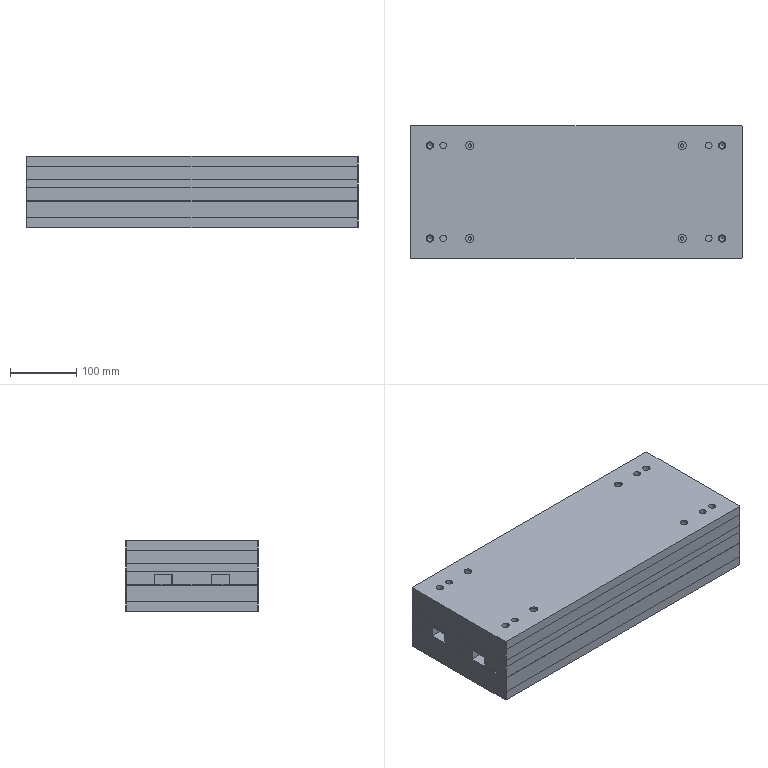Part | NX | features BREP 6 | 6 solids | 1558 faces | box 500 x 200 x 107.6 mm | volume 9875753 mm3 | plane 938 | cylinder 608 | cone 12 | commonest cylinder face diameters 1 x92 1.1 x69 1.05 x65 1.2 x65 0.8 x46 0.9 x46